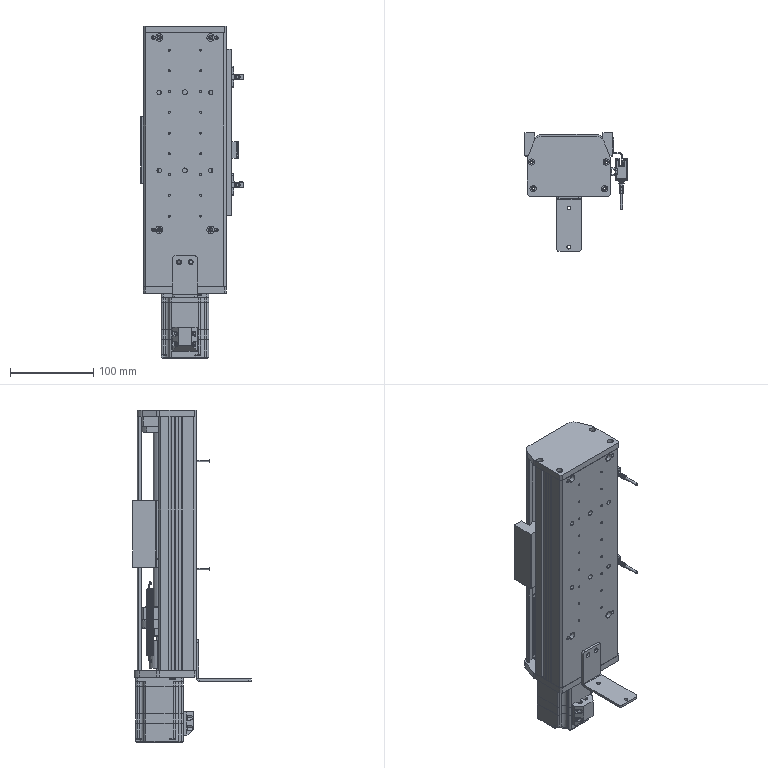Part | SolidWorks | features LocalLPattern 2, ReferencePattern 2, CompositeCurve 1 | 39 solids | 4661 faces | volume 1242766 mm3 | plane 1579 | cone 1441 | cylinder 1158 | spline 417 | torus 42 | sphere 24 | commonest cylinder face diameters 6 x112 0.4 x82 3 x78 2.5 x74 3.3 x68 0.6 x63